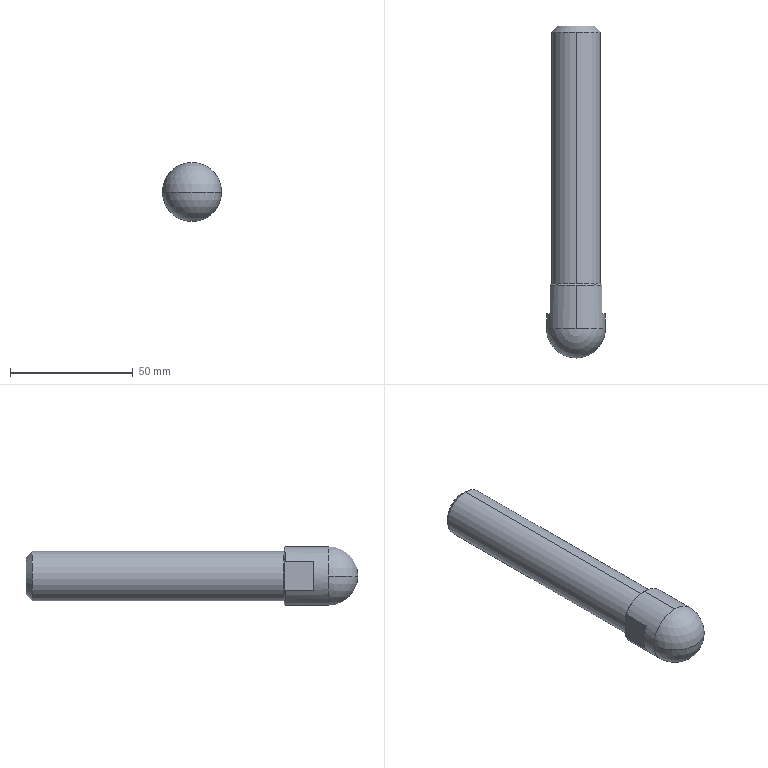Part | NX | features BREP 1 | 1 solid | 19 faces | box 24 x 135 x 24 mm | volume 44281 mm3 | plane 6 | cone 5 | cylinder 4 | torus 2 | sphere 2 | commonest cylinder face diameters 20 x2 24 x2
STEP:
#1=CARTESIAN_POINT('',(0.,-105.,10.3));
#2=VERTEX_POINT('',#1);
#3=CARTESIAN_POINT('',(0.,-105.,-10.3));
#4=VERTEX_POINT('',#3);
#5=CARTESIAN_POINT('',(0.,-105.,0.));
#6=DIRECTION('',(0.,-1.,0.));
#7=DIRECTION('',(0.,0.,-1.));
#8=AXIS2_PLACEMENT_3D('',#5,#6,#7);
#9=CIRCLE('',#8,10.3);
#10=EDGE_CURVE('',#2,#4,#9,.T.);
#11=ORIENTED_EDGE('',*,*,#10,.F.);
#12=CARTESIAN_POINT('',(0.,-104.7,10.));
#13=VERTEX_POINT('',#12);
#14=CARTESIAN_POINT('',(0.,-104.7,10.3));
#15=DIRECTION('',(1.,0.,0.));
#16=DIRECTION('',(0.,0.,-1.));
#17=AXIS2_PLACEMENT_3D('',#14,#15,#16);
#18=CIRCLE('',#17,0.3);
#19=EDGE_CURVE('',#2,#13,#18,.T.);
#20=ORIENTED_EDGE('',*,*,#19,.T.);
#21=CARTESIAN_POINT('',(0.,-104.7,-10.));
#22=VERTEX_POINT('',#21);
#23=CARTESIAN_POINT('',(0.,-104.7,0.));
#24=DIRECTION('',(0.,1.,0.));
#25=DIRECTION('',(0.,0.,-1.));
#26=AXIS2_PLACEMENT_3D('',#23,#24,#25);
#27=CIRCLE('',#26,10.);
#28=EDGE_CURVE('',#22,#13,#27,.T.);
#29=ORIENTED_EDGE('',*,*,#28,.F.);
#30=CARTESIAN_POINT('',(0.,-104.7,-10.3));
#31=DIRECTION('',(-1.,0.,0.));
#32=DIRECTION('',(0.,0.,1.));
#33=AXIS2_PLACEMENT_3D('',#30,#31,#32);
#34=CIRCLE('',#33,0.3);
#35=EDGE_CURVE('',#4,#22,#34,.T.);
#36=ORIENTED_EDGE('',*,*,#35,.F.);
#37=EDGE_LOOP('',(#11,#20,#29,#36));
#38=FACE_BOUND('',#37,.T.);
#39=CARTESIAN_POINT('',(0.,-104.7,0.));
#40=DIRECTION('',(0.,-1.,0.));
#41=DIRECTION('',(0.,0.,-1.));
#42=AXIS2_PLACEMENT_3D('',#39,#40,#41);
#43=TOROIDAL_SURFACE('',#42,10.3,0.3);
#44=ADVANCED_FACE('',(#38),#43,.F.);
#45=CARTESIAN_POINT('',(0.,0.,7.5));
#46=VERTEX_POINT('',#45);
#47=CARTESIAN_POINT('',(0.,0.,-7.5));
#48=VERTEX_POINT('',#47);
#49=CARTESIAN_POINT('',(0.,0.,0.));
#50=DIRECTION('',(0.,1.,0.));
#51=DIRECTION('',(0.,0.,-1.));
#52=AXIS2_PLACEMENT_3D('',#49,#50,#51);
#53=CIRCLE('',#52,7.5);
#54=EDGE_CURVE('',#46,#48,#53,.T.);
#55=ORIENTED_EDGE('',*,*,#54,.F.);
#56=CARTESIAN_POINT('',(0.,-2.5,10.));
#57=VERTEX_POINT('',#56);
#58=CARTESIAN_POINT('',(0.,0.,7.5));
#59=DIRECTION('',(0.,-0.7071,0.7071));
#60=VECTOR('',#59,1000.);
#61=LINE('',#58,#60);
#62=EDGE_CURVE('',#46,#57,#61,.T.);
#63=ORIENTED_EDGE('',*,*,#62,.T.);
#64=CARTESIAN_POINT('',(0.,-2.5,-10.));
#65=VERTEX_POINT('',#64);
#66=CARTESIAN_POINT('',(0.,-2.5,0.));
#67=DIRECTION('',(0.,-1.,0.));
#68=DIRECTION('',(0.,0.,-1.));
#69=AXIS2_PLACEMENT_3D('',#66,#67,#68);
#70=CIRCLE('',#69,10.);
#71=EDGE_CURVE('',#65,#57,#70,.T.);
#72=ORIENTED_EDGE('',*,*,#71,.F.);
#73=CARTESIAN_POINT('',(0.,0.,-7.5));
#74=DIRECTION('',(0.,-0.7071,-0.7071));
#75=VECTOR('',#74,1000.);
#76=LINE('',#73,#75);
#77=EDGE_CURVE('',#48,#65,#76,.T.);
#78=ORIENTED_EDGE('',*,*,#77,.F.);
#79=EDGE_LOOP('',(#55,#63,#72,#78));
#80=FACE_BOUND('',#79,.T.);
#81=CARTESIAN_POINT('',(0.,0.,0.));
#82=DIRECTION('',(0.,-1.,0.));
#83=DIRECTION('',(0.,0.,-1.));
#84=AXIS2_PLACEMENT_3D('',#81,#82,#83);
#85=CONICAL_SURFACE('',#84,7.5,0.7854);
#86=ADVANCED_FACE('',(#80),#85,.T.);
#87=CARTESIAN_POINT('',(0.,-104.7,0.));
#88=DIRECTION('',(0.,1.,0.));
#89=DIRECTION('',(0.,0.,-1.));
#90=AXIS2_PLACEMENT_3D('',#87,#88,#89);
#91=CIRCLE('',#90,10.);
#92=EDGE_CURVE('',#13,#22,#91,.T.);
#93=ORIENTED_EDGE('',*,*,#92,.T.);
#94=CARTESIAN_POINT('',(0.,0.,-10.));
#95=DIRECTION('',(0.,1.,0.));
#96=VECTOR('',#95,1000.);
#97=LINE('',#94,#96);
#98=EDGE_CURVE('',#65,#22,#97,.F.);
#99=ORIENTED_EDGE('',*,*,#98,.F.);
#100=ORIENTED_EDGE('',*,*,#71,.T.);
#101=CARTESIAN_POINT('',(0.,0.,10.));
#102=DIRECTION('',(0.,1.,0.));
#103=VECTOR('',#102,1000.);
#104=LINE('',#101,#103);
#105=EDGE_CURVE('',#57,#13,#104,.F.);
#106=ORIENTED_EDGE('',*,*,#105,.T.);
#107=EDGE_LOOP('',(#93,#99,#100,#106));
#108=FACE_BOUND('',#107,.T.);
#109=CARTESIAN_POINT('',(0.,0.,0.));
#110=DIRECTION('',(0.,1.,0.));
#111=DIRECTION('',(0.,0.,1.));
#112=AXIS2_PLACEMENT_3D('',#109,#110,#111);
#113=CYLINDRICAL_SURFACE('',#112,10.);
#114=ADVANCED_FACE('',(#108),#113,.T.);
#115=CARTESIAN_POINT('',(0.,-105.,-11.5));
#116=VERTEX_POINT('',#115);
#117=CARTESIAN_POINT('',(-10.5,-105.,-4.69));
#118=VERTEX_POINT('',#117);
#119=CARTESIAN_POINT('',(0.,-105.,0.));
#120=DIRECTION('',(0.,1.,0.));
#121=DIRECTION('',(0.,0.,-1.));
#122=AXIS2_PLACEMENT_3D('',#119,#120,#121);
#123=CIRCLE('',#122,11.5);
#124=EDGE_CURVE('',#116,#118,#123,.T.);
#125=ORIENTED_EDGE('',*,*,#124,.F.);
#126=CARTESIAN_POINT('',(0.,-105.5,-12.));
#127=VERTEX_POINT('',#126);
#128=CARTESIAN_POINT('',(0.,-105.,-11.5));
#129=DIRECTION('',(0.,-0.7071,-0.7071));
#130=VECTOR('',#129,1000.);
#131=LINE('',#128,#130);
#132=EDGE_CURVE('',#116,#127,#131,.T.);
#133=ORIENTED_EDGE('',*,*,#132,.T.);
#134=CARTESIAN_POINT('',(-10.5,-105.5,-5.809));
#135=VERTEX_POINT('',#134);
#136=CARTESIAN_POINT('',(0.,-105.5,0.));
#137=DIRECTION('',(0.,-1.,0.));
#138=DIRECTION('',(0.,0.,-1.));
#139=AXIS2_PLACEMENT_3D('',#136,#137,#138);
#140=CIRCLE('',#139,12.);
#141=EDGE_CURVE('',#135,#127,#140,.T.);
#142=ORIENTED_EDGE('',*,*,#141,.F.);
#143=CARTESIAN_POINT('',(-10.5,-105.5,-5.809));
#144=CARTESIAN_POINT('',(-10.5,-105.321,-5.441));
#145=CARTESIAN_POINT('',(-10.5,-105.154,-5.068));
#146=CARTESIAN_POINT('',(-10.5,-105.,-4.69));
#147=B_SPLINE_CURVE_WITH_KNOTS('',3,(#143,#144,#145,#146),.UNSPECIFIED.,.F.,.F.,(4,4),(0.01988,0.02111),.UNSPECIFIED.);
#148=EDGE_CURVE('',#135,#118,#147,.T.);
#149=ORIENTED_EDGE('',*,*,#148,.T.);
#150=EDGE_LOOP('',(#125,#133,#142,#149));
#151=FACE_BOUND('',#150,.T.);
#152=CARTESIAN_POINT('',(0.,-105.,0.));
#153=DIRECTION('',(0.,-1.,0.));
#154=DIRECTION('',(0.,0.,-1.));
#155=AXIS2_PLACEMENT_3D('',#152,#153,#154);
#156=CONICAL_SURFACE('',#155,11.5,0.7854);
#157=ADVANCED_FACE('',(#151),#156,.T.);
#158=CARTESIAN_POINT('',(0.,-123.,12.));
#159=VERTEX_POINT('',#158);
#160=CARTESIAN_POINT('',(12.,-123.,0.));
#161=VERTEX_POINT('',#160);
#162=CARTESIAN_POINT('',(0.,-123.,0.));
#163=DIRECTION('',(0.,1.,0.));
#164=DIRECTION('',(0.,0.,1.));
#165=AXIS2_PLACEMENT_3D('',#162,#163,#164);
#166=CIRCLE('',#165,12.);
#167=EDGE_CURVE('',#159,#161,#166,.T.);
#168=ORIENTED_EDGE('',*,*,#167,.T.);
#169=CARTESIAN_POINT('',(0.,-123.,-12.));
#170=VERTEX_POINT('',#169);
#171=CARTESIAN_POINT('',(0.,-123.,0.));
#172=DIRECTION('',(0.,1.,0.));
#173=DIRECTION('',(0.,0.,1.));
#174=AXIS2_PLACEMENT_3D('',#171,#172,#173);
#175=CIRCLE('',#174,12.);
#176=EDGE_CURVE('',#161,#170,#175,.T.);
#177=ORIENTED_EDGE('',*,*,#176,.T.);
#178=CARTESIAN_POINT('',(0.,0.,-12.));
#179=DIRECTION('',(0.,1.,0.));
#180=VECTOR('',#179,1000.);
#181=LINE('',#178,#180);
#182=EDGE_CURVE('',#127,#170,#181,.F.);
#183=ORIENTED_EDGE('',*,*,#182,.F.);
#184=CARTESIAN_POINT('',(10.5,-105.5,-5.809));
#185=VERTEX_POINT('',#184);
#186=CARTESIAN_POINT('',(0.,-105.5,0.));
#187=DIRECTION('',(0.,-1.,0.));
#188=DIRECTION('',(0.,0.,-1.));
#189=AXIS2_PLACEMENT_3D('',#186,#187,#188);
#190=CIRCLE('',#189,12.);
#191=EDGE_CURVE('',#127,#185,#190,.T.);
#192=ORIENTED_EDGE('',*,*,#191,.T.);
#193=CARTESIAN_POINT('',(10.5,-117.,-5.809));
#194=VERTEX_POINT('',#193);
#195=CARTESIAN_POINT('',(10.5,0.,-5.809));
#196=DIRECTION('',(0.,-1.,0.));
#197=VECTOR('',#196,1000.);
#198=LINE('',#195,#197);
#199=EDGE_CURVE('',#185,#194,#198,.T.);
#200=ORIENTED_EDGE('',*,*,#199,.T.);
#201=CARTESIAN_POINT('',(10.5,-117.,5.809));
#202=VERTEX_POINT('',#201);
#203=CARTESIAN_POINT('',(0.,-117.,0.));
#204=DIRECTION('',(0.,-1.,0.));
#205=DIRECTION('',(0.,0.,-1.));
#206=AXIS2_PLACEMENT_3D('',#203,#204,#205);
#207=CIRCLE('',#206,12.);
#208=EDGE_CURVE('',#194,#202,#207,.T.);
#209=ORIENTED_EDGE('',*,*,#208,.T.);
#210=CARTESIAN_POINT('',(10.5,-105.5,5.809));
#211=VERTEX_POINT('',#210);
#212=CARTESIAN_POINT('',(10.5,0.,5.809));
#213=DIRECTION('',(0.,1.,0.));
#214=VECTOR('',#213,1000.);
#215=LINE('',#212,#214);
#216=EDGE_CURVE('',#202,#211,#215,.T.);
#217=ORIENTED_EDGE('',*,*,#216,.T.);
#218=CARTESIAN_POINT('',(0.,-105.5,12.));
#219=VERTEX_POINT('',#218);
#220=CARTESIAN_POINT('',(0.,-105.5,0.));
#221=DIRECTION('',(0.,-1.,0.));
#222=DIRECTION('',(0.,0.,-1.));
#223=AXIS2_PLACEMENT_3D('',#220,#221,#222);
#224=CIRCLE('',#223,12.);
#225=EDGE_CURVE('',#211,#219,#224,.T.);
#226=ORIENTED_EDGE('',*,*,#225,.T.);
#227=CARTESIAN_POINT('',(0.,0.,12.));
#228=DIRECTION('',(0.,1.,0.));
#229=VECTOR('',#228,1000.);
#230=LINE('',#227,#229);
#231=EDGE_CURVE('',#219,#159,#230,.F.);
#232=ORIENTED_EDGE('',*,*,#231,.T.);
#233=EDGE_LOOP('',(#168,#177,#183,#192,#200,#209,#217,#226,#232));
#234=FACE_BOUND('',#233,.T.);
#235=CARTESIAN_POINT('',(0.,0.,0.));
#236=DIRECTION('',(0.,1.,0.));
#237=DIRECTION('',(0.,0.,1.));
#238=AXIS2_PLACEMENT_3D('',#235,#236,#237);
#239=CYLINDRICAL_SURFACE('',#238,12.);
#240=ADVANCED_FACE('',(#234),#239,.T.);
#241=CARTESIAN_POINT('',(-10.5,-105.,4.69));
#242=VERTEX_POINT('',#241);
#243=CARTESIAN_POINT('',(-10.5,-105.,-10.));
#244=DIRECTION('',(0.,0.,1.));
#245=VECTOR('',#244,1000.);
#246=LINE('',#243,#245);
#247=EDGE_CURVE('',#118,#242,#246,.T.);
#248=ORIENTED_EDGE('',*,*,#247,.T.);
#249=CARTESIAN_POINT('',(10.5,-105.,4.69));
#250=VERTEX_POINT('',#249);
#251=CARTESIAN_POINT('',(0.,-105.,0.));
#252=DIRECTION('',(0.,1.,0.));
#253=DIRECTION('',(0.,0.,-1.));
#254=AXIS2_PLACEMENT_3D('',#251,#252,#253);
#255=CIRCLE('',#254,11.5);
#256=EDGE_CURVE('',#242,#250,#255,.T.);
#257=ORIENTED_EDGE('',*,*,#256,.T.);
#258=CARTESIAN_POINT('',(10.5,-105.,-4.69));
#259=VERTEX_POINT('',#258);
#260=CARTESIAN_POINT('',(10.5,-105.,-10.));
#261=DIRECTION('',(0.,0.,1.));
#262=VECTOR('',#261,1000.);
#263=LINE('',#260,#262);
#264=EDGE_CURVE('',#259,#250,#263,.T.);
#265=ORIENTED_EDGE('',*,*,#264,.F.);
#266=CARTESIAN_POINT('',(0.,-105.,0.));
#267=DIRECTION('',(0.,1.,0.));
#268=DIRECTION('',(0.,0.,-1.));
#269=AXIS2_PLACEMENT_3D('',#266,#267,#268);
#270=CIRCLE('',#269,11.5);
#271=EDGE_CURVE('',#259,#116,#270,.T.);
#272=ORIENTED_EDGE('',*,*,#271,.T.);
#273=ORIENTED_EDGE('',*,*,#124,.T.);
#274=EDGE_LOOP('',(#248,#257,#265,#272,#273));
#275=FACE_BOUND('',#274,.T.);
#276=CARTESIAN_POINT('',(0.,-105.,0.));
#277=DIRECTION('',(0.,-1.,0.));
#278=DIRECTION('',(0.,0.,-1.));
#279=AXIS2_PLACEMENT_3D('',#276,#277,#278);
#280=CIRCLE('',#279,10.3);
#281=EDGE_CURVE('',#4,#2,#280,.T.);
#282=ORIENTED_EDGE('',*,*,#281,.T.);
#283=ORIENTED_EDGE('',*,*,#10,.T.);
#284=EDGE_LOOP('',(#282,#283));
#285=FACE_BOUND('',#284,.T.);
#286=CARTESIAN_POINT('',(10.,-105.,0.));
#287=DIRECTION('',(0.,-1.,0.));
#288=DIRECTION('',(0.,0.,-1.));
#289=AXIS2_PLACEMENT_3D('',#286,#287,#288);
#290=PLANE('',#289);
#291=ADVANCED_FACE('',(#275,#285),#290,.F.);
#292=ORIENTED_EDGE('',*,*,#182,.T.);
#293=CARTESIAN_POINT('',(-12.,-123.,0.));
#294=VERTEX_POINT('',#293);
#295=CARTESIAN_POINT('',(0.,-123.,0.));
#296=DIRECTION('',(0.,1.,0.));
#297=DIRECTION('',(0.,0.,1.));
#298=AXIS2_PLACEMENT_3D('',#295,#296,#297);
#299=CIRCLE('',#298,12.);
#300=EDGE_CURVE('',#170,#294,#299,.T.);
#301=ORIENTED_EDGE('',*,*,#300,.T.);
#302=CARTESIAN_POINT('',(0.,-123.,0.));
#303=DIRECTION('',(0.,1.,0.));
#304=DIRECTION('',(0.,0.,1.));
#305=AXIS2_PLACEMENT_3D('',#302,#303,#304);
#306=CIRCLE('',#305,12.);
#307=EDGE_CURVE('',#294,#159,#306,.T.);
#308=ORIENTED_EDGE('',*,*,#307,.T.);
#309=ORIENTED_EDGE('',*,*,#231,.F.);
#310=CARTESIAN_POINT('',(-10.5,-105.5,5.809));
#311=VERTEX_POINT('',#310);
#312=CARTESIAN_POINT('',(0.,-105.5,0.));
#313=DIRECTION('',(0.,-1.,0.));
#314=DIRECTION('',(0.,0.,-1.));
#315=AXIS2_PLACEMENT_3D('',#312,#313,#314);
#316=CIRCLE('',#315,12.);
#317=EDGE_CURVE('',#219,#311,#316,.T.);
#318=ORIENTED_EDGE('',*,*,#317,.T.);
#319=CARTESIAN_POINT('',(-10.5,-117.,5.809));
#320=VERTEX_POINT('',#319);
#321=CARTESIAN_POINT('',(-10.5,0.,5.809));
#322=DIRECTION('',(0.,1.,0.));
#323=VECTOR('',#322,1000.);
#324=LINE('',#321,#323);
#325=EDGE_CURVE('',#320,#311,#324,.T.);
#326=ORIENTED_EDGE('',*,*,#325,.F.);
#327=CARTESIAN_POINT('',(-10.5,-117.,-5.809));
#328=VERTEX_POINT('',#327);
#329=CARTESIAN_POINT('',(0.,-117.,0.));
#330=DIRECTION('',(0.,1.,0.));
#331=DIRECTION('',(0.,0.,1.));
#332=AXIS2_PLACEMENT_3D('',#329,#330,#331);
#333=CIRCLE('',#332,12.);
#334=EDGE_CURVE('',#328,#320,#333,.T.);
#335=ORIENTED_EDGE('',*,*,#334,.F.);
#336=CARTESIAN_POINT('',(-10.5,0.,-5.809));
#337=DIRECTION('',(0.,-1.,0.));
#338=VECTOR('',#337,1000.);
#339=LINE('',#336,#338);
#340=EDGE_CURVE('',#135,#328,#339,.T.);
#341=ORIENTED_EDGE('',*,*,#340,.F.);
#342=ORIENTED_EDGE('',*,*,#141,.T.);
#343=EDGE_LOOP('',(#292,#301,#308,#309,#318,#326,#335,#341,#342));
#344=FACE_BOUND('',#343,.T.);
#345=CARTESIAN_POINT('',(0.,0.,0.));
#346=DIRECTION('',(0.,1.,0.));
#347=DIRECTION('',(0.,0.,1.));
#348=AXIS2_PLACEMENT_3D('',#345,#346,#347);
#349=CYLINDRICAL_SURFACE('',#348,12.);
#350=ADVANCED_FACE('',(#344),#349,.T.);
#351=ORIENTED_EDGE('',*,*,#132,.F.);
#352=ORIENTED_EDGE('',*,*,#271,.F.);
#353=CARTESIAN_POINT('',(10.5,-105.5,-5.809));
#354=CARTESIAN_POINT('',(10.5,-105.321,-5.441));
#355=CARTESIAN_POINT('',(10.5,-105.154,-5.068));
#356=CARTESIAN_POINT('',(10.5,-105.,-4.69));
#357=B_SPLINE_CURVE_WITH_KNOTS('',3,(#353,#354,#355,#356),.UNSPECIFIED.,.F.,.F.,(4,4),(0.01988,0.02111),.UNSPECIFIED.);
#358=EDGE_CURVE('',#185,#259,#357,.T.);
#359=ORIENTED_EDGE('',*,*,#358,.F.);
#360=ORIENTED_EDGE('',*,*,#191,.F.);
#361=EDGE_LOOP('',(#351,#352,#359,#360));
#362=FACE_BOUND('',#361,.T.);
#363=CARTESIAN_POINT('',(0.,-105.,0.));
#364=DIRECTION('',(0.,-1.,0.));
#365=DIRECTION('',(0.,0.,-1.));
#366=AXIS2_PLACEMENT_3D('',#363,#364,#365);
#367=CONICAL_SURFACE('',#366,11.5,0.7854);
#368=ADVANCED_FACE('',(#362),#367,.T.);
#369=ORIENTED_EDGE('',*,*,#256,.F.);
#370=CARTESIAN_POINT('',(-10.5,-105.,4.69));
#371=CARTESIAN_POINT('',(-10.5,-105.154,5.068));
#372=CARTESIAN_POINT('',(-10.5,-105.321,5.441));
#373=CARTESIAN_POINT('',(-10.5,-105.5,5.809));
#374=B_SPLINE_CURVE_WITH_KNOTS('',3,(#370,#371,#372,#373),.UNSPECIFIED.,.F.,.F.,(4,4),(0.03076,0.03199),.UNSPECIFIED.);
#375=EDGE_CURVE('',#242,#311,#374,.T.);
#376=ORIENTED_EDGE('',*,*,#375,.T.);
#377=ORIENTED_EDGE('',*,*,#317,.F.);
#378=ORIENTED_EDGE('',*,*,#225,.F.);
#379=CARTESIAN_POINT('',(10.5,-105.,4.69));
#380=CARTESIAN_POINT('',(10.5,-105.154,5.068));
#381=CARTESIAN_POINT('',(10.5,-105.321,5.441));
#382=CARTESIAN_POINT('',(10.5,-105.5,5.809));
#383=B_SPLINE_CURVE_WITH_KNOTS('',3,(#379,#380,#381,#382),.UNSPECIFIED.,.F.,.F.,(4,4),(0.03076,0.03199),.UNSPECIFIED.);
#384=EDGE_CURVE('',#250,#211,#383,.T.);
#385=ORIENTED_EDGE('',*,*,#384,.F.);
#386=EDGE_LOOP('',(#369,#376,#377,#378,#385));
#387=FACE_BOUND('',#386,.T.);
#388=CARTESIAN_POINT('',(0.,-105.,0.));
#389=DIRECTION('',(0.,-1.,0.));
#390=DIRECTION('',(0.,0.,-1.));
#391=AXIS2_PLACEMENT_3D('',#388,#389,#390);
#392=CONICAL_SURFACE('',#391,11.5,0.7854);
#393=ADVANCED_FACE('',(#387),#392,.T.);
#394=CARTESIAN_POINT('',(0.,0.,0.));
#395=DIRECTION('',(0.,1.,0.));
#396=DIRECTION('',(0.,0.,-1.));
#397=AXIS2_PLACEMENT_3D('',#394,#395,#396);
#398=CIRCLE('',#397,7.5);
#399=EDGE_CURVE('',#48,#46,#398,.T.);
#400=ORIENTED_EDGE('',*,*,#399,.T.);
#401=ORIENTED_EDGE('',*,*,#54,.T.);
#402=EDGE_LOOP('',(#400,#401));
#403=FACE_BOUND('',#402,.T.);
#404=CARTESIAN_POINT('',(0.,0.,0.));
#405=DIRECTION('',(0.,-1.,0.));
#406=DIRECTION('',(0.,0.,-1.));
#407=AXIS2_PLACEMENT_3D('',#404,#405,#406);
#408=PLANE('',#407);
#409=ADVANCED_FACE('',(#403),#408,.F.);
#410=ORIENTED_EDGE('',*,*,#98,.T.);
#411=ORIENTED_EDGE('',*,*,#28,.T.);
#412=ORIENTED_EDGE('',*,*,#105,.F.);
#413=CARTESIAN_POINT('',(0.,-2.5,0.));
#414=DIRECTION('',(0.,-1.,0.));
#415=DIRECTION('',(0.,0.,-1.));
#416=AXIS2_PLACEMENT_3D('',#413,#414,#415);
#417=CIRCLE('',#416,10.);
#418=EDGE_CURVE('',#57,#65,#417,.T.);
#419=ORIENTED_EDGE('',*,*,#418,.T.);
#420=EDGE_LOOP('',(#410,#411,#412,#419));
#421=FACE_BOUND('',#420,.T.);
#422=CARTESIAN_POINT('',(0.,0.,0.));
#423=DIRECTION('',(0.,1.,0.));
#424=DIRECTION('',(0.,0.,1.));
#425=AXIS2_PLACEMENT_3D('',#422,#423,#424);
#426=CYLINDRICAL_SURFACE('',#425,10.);
#427=ADVANCED_FACE('',(#421),#426,.T.);
#428=CARTESIAN_POINT('',(0.,-135.,0.));
#429=VERTEX_POINT('',#428);
#430=CARTESIAN_POINT('',(0.,-123.,0.));
#431=DIRECTION('',(0.,0.,-1.));
#432=DIRECTION('',(-1.,0.,0.));
#433=AXIS2_PLACEMENT_3D('',#430,#431,#432);
#434=CIRCLE('',#433,12.);
#435=EDGE_CURVE('',#429,#294,#434,.T.);
#436=ORIENTED_EDGE('',*,*,#435,.F.);
#437=CARTESIAN_POINT('',(0.,-123.,0.));
#438=DIRECTION('',(0.,0.,1.));
#439=DIRECTION('',(1.,0.,0.));
#440=AXIS2_PLACEMENT_3D('',#437,#438,#439);
#441=CIRCLE('',#440,12.);
#442=EDGE_CURVE('',#429,#161,#441,.T.);
#443=ORIENTED_EDGE('',*,*,#442,.T.);
#444=ORIENTED_EDGE('',*,*,#167,.F.);
#445=ORIENTED_EDGE('',*,*,#307,.F.);
#446=EDGE_LOOP('',(#436,#443,#444,#445));
#447=FACE_BOUND('',#446,.T.);
#448=CARTESIAN_POINT('',(0.,-123.,0.));
#449=DIRECTION('',(0.,0.,-1.));
#450=DIRECTION('',(1.,0.,0.));
#451=AXIS2_PLACEMENT_3D('',#448,#449,#450);
#452=SPHERICAL_SURFACE('',#451,12.);
#453=ADVANCED_FACE('',(#447),#452,.T.);
#454=ORIENTED_EDGE('',*,*,#62,.F.);
#455=ORIENTED_EDGE('',*,*,#399,.F.);
#456=ORIENTED_EDGE('',*,*,#77,.T.);
#457=ORIENTED_EDGE('',*,*,#418,.F.);
#458=EDGE_LOOP('',(#454,#455,#456,#457));
#459=FACE_BOUND('',#458,.T.);
#460=CARTESIAN_POINT('',(0.,0.,0.));
#461=DIRECTION('',(0.,-1.,0.));
#462=DIRECTION('',(0.,0.,-1.));
#463=AXIS2_PLACEMENT_3D('',#460,#461,#462);
#464=CONICAL_SURFACE('',#463,7.5,0.7854);
#465=ADVANCED_FACE('',(#459),#464,.T.);
#466=ORIENTED_EDGE('',*,*,#19,.F.);
#467=ORIENTED_EDGE('',*,*,#281,.F.);
#468=ORIENTED_EDGE('',*,*,#35,.T.);
#469=ORIENTED_EDGE('',*,*,#92,.F.);
#470=EDGE_LOOP('',(#466,#467,#468,#469));
#471=FACE_BOUND('',#470,.T.);
#472=CARTESIAN_POINT('',(0.,-104.7,0.));
#473=DIRECTION('',(0.,-1.,0.));
#474=DIRECTION('',(0.,0.,-1.));
#475=AXIS2_PLACEMENT_3D('',#472,#473,#474);
#476=TOROIDAL_SURFACE('',#475,10.3,0.3);
#477=ADVANCED_FACE('',(#471),#476,.F.);
#478=CARTESIAN_POINT('',(10.5,-117.,-10.));
#479=DIRECTION('',(0.,0.,1.));
#480=VECTOR('',#479,1000.);
#481=LINE('',#478,#480);
#482=EDGE_CURVE('',#194,#202,#481,.T.);
#483=ORIENTED_EDGE('',*,*,#482,.T.);
#484=ORIENTED_EDGE('',*,*,#208,.F.);
#485=EDGE_LOOP('',(#483,#484));
#486=FACE_BOUND('',#485,.T.);
#487=CARTESIAN_POINT('',(10.5,-117.,-10.));
#488=DIRECTION('',(0.,-1.,0.));
#489=DIRECTION('',(0.,0.,-1.));
#490=AXIS2_PLACEMENT_3D('',#487,#488,#489);
#491=PLANE('',#490);
#492=ADVANCED_FACE('',(#486),#491,.F.);
#493=ORIENTED_EDGE('',*,*,#358,.T.);
#494=ORIENTED_EDGE('',*,*,#264,.T.);
#495=ORIENTED_EDGE('',*,*,#384,.T.);
#496=ORIENTED_EDGE('',*,*,#216,.F.);
#497=ORIENTED_EDGE('',*,*,#482,.F.);
#498=ORIENTED_EDGE('',*,*,#199,.F.);
#499=EDGE_LOOP('',(#493,#494,#495,#496,#497,#498));
#500=FACE_BOUND('',#499,.T.);
#501=CARTESIAN_POINT('',(10.5,-105.,-10.));
#502=DIRECTION('',(-1.,0.,0.));
#503=DIRECTION('',(0.,1.,0.));
#504=AXIS2_PLACEMENT_3D('',#501,#502,#503);
#505=PLANE('',#504);
#506=ADVANCED_FACE('',(#500),#505,.F.);
#507=ORIENTED_EDGE('',*,*,#334,.T.);
#508=CARTESIAN_POINT('',(-10.5,-117.,-10.));
#509=DIRECTION('',(0.,0.,1.));
#510=VECTOR('',#509,1000.);
#511=LINE('',#508,#510);
#512=EDGE_CURVE('',#328,#320,#511,.T.);
#513=ORIENTED_EDGE('',*,*,#512,.F.);
#514=EDGE_LOOP('',(#507,#513));
#515=FACE_BOUND('',#514,.T.);
#516=CARTESIAN_POINT('',(-10.5,-117.,-10.));
#517=DIRECTION('',(0.,1.,0.));
#518=DIRECTION('',(1.,0.,0.));
#519=AXIS2_PLACEMENT_3D('',#516,#517,#518);
#520=PLANE('',#519);
#521=ADVANCED_FACE('',(#515),#520,.T.);
#522=ORIENTED_EDGE('',*,*,#340,.T.);
#523=ORIENTED_EDGE('',*,*,#512,.T.);
#524=ORIENTED_EDGE('',*,*,#325,.T.);
#525=ORIENTED_EDGE('',*,*,#375,.F.);
#526=ORIENTED_EDGE('',*,*,#247,.F.);
#527=ORIENTED_EDGE('',*,*,#148,.F.);
#528=EDGE_LOOP('',(#522,#523,#524,#525,#526,#527));
#529=FACE_BOUND('',#528,.T.);
#530=CARTESIAN_POINT('',(-10.5,-105.,-10.));
#531=DIRECTION('',(-1.,0.,0.));
#532=DIRECTION('',(0.,0.,1.));
#533=AXIS2_PLACEMENT_3D('',#530,#531,#532);
#534=PLANE('',#533);
#535=ADVANCED_FACE('',(#529),#534,.T.);
#536=ORIENTED_EDGE('',*,*,#442,.F.);
#537=ORIENTED_EDGE('',*,*,#435,.T.);
#538=ORIENTED_EDGE('',*,*,#300,.F.);
#539=ORIENTED_EDGE('',*,*,#176,.F.);
#540=EDGE_LOOP('',(#536,#537,#538,#539));
#541=FACE_BOUND('',#540,.T.);
#542=CARTESIAN_POINT('',(0.,-123.,0.));
#543=DIRECTION('',(0.,0.,-1.));
#544=DIRECTION('',(1.,0.,0.));
#545=AXIS2_PLACEMENT_3D('',#542,#543,#544);
#546=SPHERICAL_SURFACE('',#545,12.);
#547=ADVANCED_FACE('',(#541),#546,.T.);
#548=CLOSED_SHELL('',(#44,#86,#114,#157,#240,#291,#350,#368,#393,#409,#427,#453,#465,#477,#492,#506,#521,#535,#547));
#549=MANIFOLD_SOLID_BREP('',#548);
#550=(LENGTH_UNIT()NAMED_UNIT(*)SI_UNIT(.MILLI.,.METRE.));
#551=UNCERTAINTY_MEASURE_WITH_UNIT(LENGTH_MEASURE(0.00001),#550,'','');
#552=(NAMED_UNIT(*)PLANE_ANGLE_UNIT()SI_UNIT($,.RADIAN.));
#553=(NAMED_UNIT(*)SI_UNIT($,.STERADIAN.)SOLID_ANGLE_UNIT());
#554=(GEOMETRIC_REPRESENTATION_CONTEXT(3)GLOBAL_UNCERTAINTY_ASSIGNED_CONTEXT((#551))GLOBAL_UNIT_ASSIGNED_CONTEXT((#550,#552,#553))REPRESENTATION_CONTEXT('',''));
#555=ADVANCED_BREP_SHAPE_REPRESENTATION('',(#549),#554);